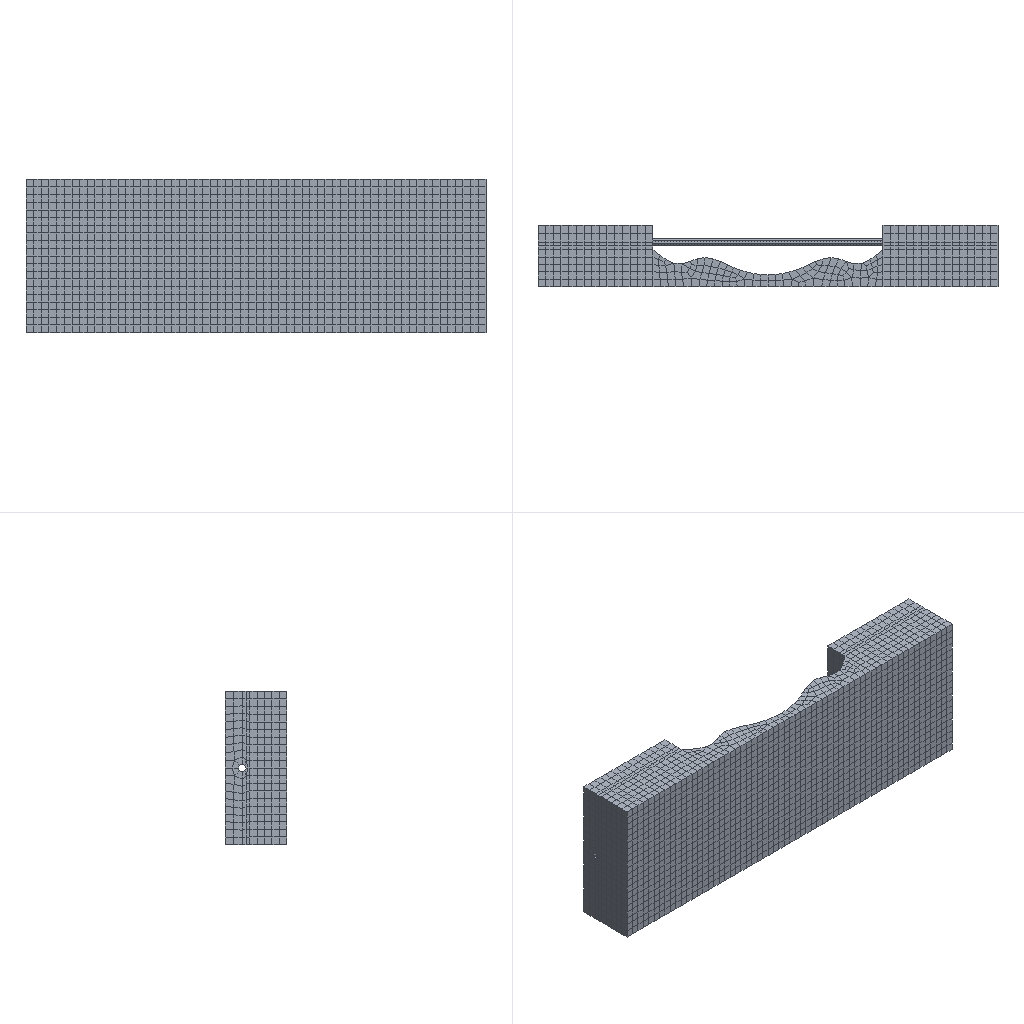Simulation study | abaqus
Set-up summary:
category,name,step,type,value,unit,region
solver,abaqus
solver,version,,,Abaqus/Standard 2020
units,not stated in the deck,,not stated
analysis,deck,,static,static
load_step,Step-G,Step-G,static,nlgeom=True
load_step,Step-2,Step-2,static,nlgeom=True
load_step,Step-3,Step-3,static,nlgeom=True
load_step,Step-4,Step-4,static,nlgeom=True
contact,interactions,,,general=1 pairs=0 ties=0
load_step,requested,,,4
mesh,nodes,,,11095
mesh,elements,,,9024
element_type,S4R,,shell,1224
element_type,C3D8R,,solid,7800
load,load commands in deck,,count,5
bc,support commands in deck,,count,4
material,GUANDAO,,in results
material,HAI,,in results
check,setup vs results,,match,"per instance, exact: element labels, types and connectivity; labels of the nodes the elements use; coordinates not compared"
Abaqus input file, long lists of numbers shortened:
*Heading
** Job name: Job-1 Model name: Model-1
** Generated by: Abaqus/CAE 2020
*Preprint, echo=NO, model=NO, history=NO, contact=NO
**
** PARTS
**
*Part, name=guan-final
*Node
      1, -0.1118, -0.2236,          30.
      2,  -0.2372, -0.07906,          30.
** (1230 more lines like these left out)
*Element, type=S4R
   1,    8,    1,    9,   16
   2,    1,    2,   10,    9
** (1222 more lines like these left out)
*Nset, nset=Set-1, generate
    1,  1232,     1
*Elset, elset=Set-1, generate
    1,  1224,     1
** Section: guandao
*Shell Section, elset=Set-1, material=guandao
0.01, 5
*End Part
**
*Part, name=merge
*Node
      1,          7.5,           0.,           5.
      2,          15.,           0.,           5.
** (9861 more lines like these left out)
*Element, type=C3D8R
  1, 1155,   96, 1141, 5340,   81,    1,   82, 1015
  2, 5340, 1141, 1142, 5341, 1015,   82,   83, 1016
** (7798 more lines like these left out)
*Nset, nset=Set-1, generate
    1,  9863,     1
*Elset, elset=Set-1, generate
    1,  7800,     1
** Section: haichuang
*Solid Section, elset=Set-1, material=hai
,
*End Part
**
**
** ASSEMBLY
**
*Assembly, name=Assembly
**
*Instance, name=merge-1, part=merge
*End Instance
**
*Instance, name=guan-final-1, part=guan-final
        -15.,          0.5,           5.
        -15.,          0.5,           5.,         -15., 1.5,           5., 90.
*End Instance
**
*Nset, nset=Set-1, instance=merge-1
   19,   20,   21,   22,   39,   42,   43,   46,   49,   50,   61,   62,   68,   72,  265,  266
  267,  268,  269,  270,  271,  272,  273,  274,  275,  276,  277,  278,  279,  280,  281,  282
** (79 more lines like these left out)
*Elset, elset=Set-1, instance=merge-1
  631,  632,  633,  634,  635,  636,  637,  638,  639,  640,  641,  642,  643,  644,  645,  646
  647,  648,  649,  650,  651,  652,  653,  654,  655,  656,  657,  658,  659,  660,  661,  662
** (73 more lines like these left out)
*Nset, nset=Set-2, instance=guan-final-1
    1,    2,    3,    4,    5,    6,    7,    8, 1225, 1226, 1227, 1228, 1229, 1230, 1231, 1232
*Elset, elset=Set-2, instance=guan-final-1
    1,    2,    3,    4,    5,    6,    7,    8, 1217, 1218, 1219, 1220, 1221, 1222, 1223, 1224
*Nset, nset=Set-3, instance=merge-1
    2,    3,    5,    9,   10,   12,   16,   17,   18,   19,   22,   25,   26,   28,   30,   31
   34,   36,   38,   41,   42,   45,   46,   48,   49,   51,   54,   56,   57,   60,   61,   64
** (26 more lines like these left out)
*Elset, elset=Set-3, instance=merge-1
   15,   16,   17,   18,   19,   20,   21,   22,   23,   24,  158,  236,  244,  252,  260,  268
  276,  284,  292,  300,  308,  337,  338,  479,  487,  488,  489,  490,  491,  492,  493,  494
** (21 more lines like these left out)
*Nset, nset=Set-4, instance=merge-1
    3,    4,    7,    9,   14,   15,   17,   18,   21,   22,   27,   28,   31,   32,   37,   38
   43,   44,   45,   46,   47,   48,   49,   50,   53,   54,   57,   58,   61,   62,   63,   64
** (56 more lines like these left out)
*Elset, elset=Set-4, instance=merge-1
   24,   33,   42,   51,   60,   69,   78,   87,   88,   89,   90,   91,   92,   93,   94,  166
  175,  184,  193,  202,  211,  220,  236,  237,  238,  239,  240,  241,  242,  243,  361,  370
** (46 more lines like these left out)
*Elset, elset=_Surf-3_SNEG, internal, instance=guan-final-1, generate
    1,  1224,     1
*Surface, type=ELEMENT, name=Surf-3
_Surf-3_SNEG, SNEG
*Elset, elset=_Surf-4_S3, internal, instance=merge-1
    1,   16,   17,   18,   19,   20,   21,   22,   23,   24,   88,   89,   90,   91,   92,   93
   94,  151,  152,  153,  154,  155,  156,  157,  158,  159,  166,  175,  184,  193,  202,  211
** (52 more lines like these left out)
*Elset, elset=_Surf-4_S4, internal, instance=merge-1
   15,   24,   33,   42,   51,   60,   69,   78,   87,   94,  101,  108,  115,  122,  129,  136
  143,  150,  158,  159,  160,  161,  162,  163,  164,  165,  229,  230,  231,  232,  233,  234
** (50 more lines like these left out)
*Elset, elset=_Surf-4_S2, internal, instance=merge-1
  166,  167,  168,  169,  170,  171,  172,  173,  174,  229,  236,  237,  238,  239,  240,  241
  242,  243,  346,  353,  354,  355,  356,  357,  358,  359,  360,  361,  416,  417,  418,  419
** (52 more lines like these left out)
*Elset, elset=_Surf-4_S6, internal, instance=merge-1
  631,  646,  661,  676,  691,  706,  721,  736,  751,  766,  781,  796,  811,  826,  841,  856
  871,  886,  901,  916,  931,  946,  961,  976,  991, 1006, 1021, 1036, 1051, 1066, 1081, 1096
** (44 more lines like these left out)
*Elset, elset=_Surf-4_S5, internal, instance=merge-1
  766,  767,  768,  769,  770,  771,  772,  773,  774,  775,  776,  777,  778,  779,  780,  916
  917,  918,  919,  920,  921,  922,  923,  924,  925,  926,  927,  928,  929,  930, 1066, 1067
** (32 more lines like these left out)
*Elset, elset=_Surf-4_S1, internal, instance=merge-1
 3436, 3437, 3438, 3439, 3440, 3441, 3442, 3443, 3444, 3445, 3446, 3447, 3448, 3449, 3450, 3451
 3452, 3453, 3454, 3455, 3456, 3457, 3458, 3459, 3460, 3461, 3462, 3463, 3464, 3465, 3466, 3467
** (10 more lines like these left out)
*Elset, elset=_Surf-4_SPOS, internal, instance=guan-final-1, generate
    1,  1224,     1
*Surface, type=ELEMENT, name=Surf-4
_Surf-4_S3, S3
_Surf-4_S4, S4
_Surf-4_S2, S2
_Surf-4_S6, S6
_Surf-4_S5, S5
_Surf-4_SPOS, SPOS
_Surf-4_S1, S1
*Elset, elset=_Surf-5_S3, internal, instance=merge-1
    1,   16,   17,   18,   19,   20,   21,   22,   23,   24,   88,   89,   90,   91,   92,   93
   94,  151,  152,  153,  154,  155,  156,  157,  158,  159,  166,  175,  184,  193,  202,  211
** (52 more lines like these left out)
*Elset, elset=_Surf-5_S4, internal, instance=merge-1
   15,   24,   33,   42,   51,   60,   69,   78,   87,   94,  101,  108,  115,  122,  129,  136
  143,  150,  158,  159,  160,  161,  162,  163,  164,  165,  229,  230,  231,  232,  233,  234
** (50 more lines like these left out)
*Elset, elset=_Surf-5_S2, internal, instance=merge-1
  166,  167,  168,  169,  170,  171,  172,  173,  174,  229,  236,  237,  238,  239,  240,  241
  242,  243,  346,  353,  354,  355,  356,  357,  358,  359,  360,  361,  416,  417,  418,  419
** (52 more lines like these left out)
*Elset, elset=_Surf-5_S6, internal, instance=merge-1
  631,  646,  661,  676,  691,  706,  721,  736,  751,  766,  781,  796,  811,  826,  841,  856
  871,  886,  901,  916,  931,  946,  961,  976,  991, 1006, 1021, 1036, 1051, 1066, 1081, 1096
** (44 more lines like these left out)
*Elset, elset=_Surf-5_S5, internal, instance=merge-1
  766,  767,  768,  769,  770,  771,  772,  773,  774,  775,  776,  777,  778,  779,  780,  916
  917,  918,  919,  920,  921,  922,  923,  924,  925,  926,  927,  928,  929,  930, 1066, 1067
** (32 more lines like these left out)
*Elset, elset=_Surf-5_S1, internal, instance=merge-1
 3436, 3437, 3438, 3439, 3440, 3441, 3442, 3443, 3444, 3445, 3446, 3447, 3448, 3449, 3450, 3451
 3452, 3453, 3454, 3455, 3456, 3457, 3458, 3459, 3460, 3461, 3462, 3463, 3464, 3465, 3466, 3467
** (10 more lines like these left out)
*Elset, elset=_Surf-5_SPOS, internal, instance=guan-final-1, generate
    1,  1224,     1
*Surface, type=ELEMENT, name=Surf-5
_Surf-5_S3, S3
_Surf-5_S4, S4
_Surf-5_S2, S2
_Surf-5_S6, S6
_Surf-5_S5, S5
_Surf-5_SPOS, SPOS
_Surf-5_S1, S1
*Elset, elset=_Surf-6_SPOS, internal, instance=guan-final-1, generate
    1,  1224,     1
*Surface, type=ELEMENT, name=Surf-6
_Surf-6_SPOS, SPOS
*Elset, elset=_m_Surf-1_SPOS, internal, instance=guan-final-1, generate
    1,  1224,     1
*Surface, type=ELEMENT, name=m_Surf-1
_m_Surf-1_SPOS, SPOS
*Elset, elset=_s_Surf-1_S3, internal, instance=merge-1
  151,  152,  153,  154,  155,  156,  157,  158,  316,  317,  318,  319,  320,  321,  322,  346
  347,  348,  349,  350,  351,  352, 1397, 1398, 1399, 1400, 1401, 1402, 1403, 1626, 1627, 1628
** (3 more lines like these left out)
*Elset, elset=_s_Surf-1_S4, internal, instance=merge-1
  159,  160,  161,  162,  163,  164,  165,  229,  230,  231,  232,  233,  234,  235,  308,  309
  310,  311,  312,  313,  314,  315,  338,  339,  340,  341,  342,  343,  344,  345, 1389, 1390
** (5 more lines like these left out)
*Elset, elset=_s_Surf-1_S2, internal, instance=merge-1
  479,  480,  481,  482,  483,  484,  485,  486, 1846, 1847, 1848, 1849, 1850, 1851, 1852, 1853
 1854, 1855, 1856, 1857, 1858, 1859, 1860, 3661, 3662, 3663, 3664, 3665, 3666, 3667, 3668, 3669
** (3 more lines like these left out)
*Surface, type=ELEMENT, name=s_Surf-1
_s_Surf-1_S3, S3
_s_Surf-1_S4, S4
_s_Surf-1_S2, S2
*Elset, elset=__Int-2_gcs0_4_S3, internal, instance=merge-1, generate
 151,  158,    1
*Elset, elset=__Int-2_gcs0_4_S4, internal, instance=merge-1
 159, 160, 161, 162, 163, 164, 165, 229, 230, 231, 232, 233, 234, 235, 308, 309
 310, 311, 312, 313, 314, 315
*Surface, type=ELEMENT, name=_Int-2_gcs0_4, internal
__Int-2_gcs0_4_S3, S3
__Int-2_gcs0_4_S4, S4
*Elset, elset=__Int-2_gcs0_12_S4, internal, instance=merge-1
 1389, 1390, 1391, 1392, 1393, 1394, 1395, 1396, 1555, 1556, 1557, 1558, 1559, 1560, 1561, 1562
*Elset, elset=__Int-2_gcs0_12_S3, internal, instance=merge-1
 1397, 1398, 1399, 1400, 1401, 1402, 1403, 1626, 1627, 1628, 1629, 1630, 1631, 1632
*Surface, type=ELEMENT, name=_Int-2_gcs0_12, internal
__Int-2_gcs0_12_S4, S4
__Int-2_gcs0_12_S3, S3
*Elset, elset=__Int-2_gcs0_22_S4, internal, instance=merge-1
 4291, 4292, 4293, 4294, 4295, 4296, 4297, 4369, 4370, 4371, 4372, 4373, 4374, 4375, 4448, 4449
 4450, 4451, 4452, 4453, 4454, 4455
*Elset, elset=__Int-2_gcs0_22_S3, internal, instance=merge-1, generate
 4298,  4305,     1
*Surface, type=ELEMENT, name=_Int-2_gcs0_22, internal
__Int-2_gcs0_22_S4, S4
__Int-2_gcs0_22_S3, S3
*Elset, elset=__Int-2_gcs0_26_S4, internal, instance=merge-1, generate
 1696,  1703,     1
*Elset, elset=__Int-2_gcs0_26_S3, internal, instance=merge-1, generate
 1704,  1710,     1
*Elset, elset=__Int-2_gcs0_26_S2, internal, instance=merge-1, generate
 1846,  1860,     1
*Surface, type=ELEMENT, name=_Int-2_gcs0_26, internal
__Int-2_gcs0_26_S4, S4
__Int-2_gcs0_26_S3, S3
__Int-2_gcs0_26_S2, S2
*Elset, elset=__Int-2_gcs0_36_S3, internal, instance=merge-1
 316, 317, 318, 319, 320, 321, 322, 346, 347, 348, 349, 350, 351, 352
*Elset, elset=__Int-2_gcs0_36_S4, internal, instance=merge-1, generate
 338,  345,    1
*Elset, elset=__Int-2_gcs0_36_S2, internal, instance=merge-1, generate
 479,  486,    1
*Surface, type=ELEMENT, name=_Int-2_gcs0_36, internal
__Int-2_gcs0_36_S3, S3
__Int-2_gcs0_36_S4, S4
__Int-2_gcs0_36_S2, S2
*Elset, elset=__Int-2_gcs0_40_S3, internal, instance=merge-1, generate
 5206,  5212,     1
*Elset, elset=__Int-2_gcs0_40_S4, internal, instance=merge-1, generate
 5213,  5220,     1
*Elset, elset=__Int-2_gcs0_40_S2, internal, instance=merge-1, generate
 5236,  5250,     1
*Surface, type=ELEMENT, name=_Int-2_gcs0_40, internal
__Int-2_gcs0_40_S3, S3
__Int-2_gcs0_40_S4, S4
__Int-2_gcs0_40_S2, S2
*Elset, elset=__Int-2_gcs0_51_S3, internal, instance=merge-1, generate
 3511,  3517,     1
*Elset, elset=__Int-2_gcs0_51_S4, internal, instance=merge-1, generate
 3518,  3525,     1
*Elset, elset=__Int-2_gcs0_51_S2, internal, instance=merge-1, generate
 3661,  3675,     1
*Surface, type=ELEMENT, name=_Int-2_gcs0_51, internal
__Int-2_gcs0_51_S3, S3
__Int-2_gcs0_51_S4, S4
__Int-2_gcs0_51_S2, S2
*Elset, elset=__Int-2_gcs0_52_S4, internal, instance=merge-1, generate
 4096,  4103,     1
*Elset, elset=__Int-2_gcs0_52_S3, internal, instance=merge-1, generate
 4104,  4110,     1
*Elset, elset=__Int-2_gcs0_52_S2, internal, instance=merge-1, generate
 4111,  4125,     1
*Surface, type=ELEMENT, name=_Int-2_gcs0_52, internal
__Int-2_gcs0_52_S4, S4
__Int-2_gcs0_52_S3, S3
__Int-2_gcs0_52_S2, S2
*Elset, elset=__Int-2_gcs0_69_S4, internal, instance=merge-1
 5526, 5527, 5529, 5546, 5581, 5640, 5641, 5643, 5660, 5695, 5754, 5755, 5757, 5774, 5809, 5868
 5869, 5871, 5888, 5923, 5982, 5983, 5985, 6002, 6037, 6096, 6097, 6099, 6116, 6151, 6210, 6211
** (5 more lines like these left out)
*Elset, elset=__Int-2_gcs0_69_S6, internal, instance=merge-1
 5530, 5531, 5542, 5543, 5545, 5578, 5584, 5644, 5645, 5656, 5657, 5659, 5692, 5698, 5758, 5759
 5770, 5771, 5773, 5806, 5812, 5872, 5873, 5884, 5885, 5887, 5920, 5926, 5986, 5987, 5998, 5999
** (7 more lines like these left out)
*Surface, type=ELEMENT, name=_Int-2_gcs0_69, internal
__Int-2_gcs0_69_S4, S4
__Int-2_gcs0_69_S6, S6
*Elset, elset=__Int-2_gcs0_73_SPOS, internal, instance=guan-final-1, generate
    1,  1224,     1
*Surface, type=ELEMENT, name=_Int-2_gcs0_73, internal
__Int-2_gcs0_73_SPOS, SPOS
*Elset, elset=__Int-2_gcs0_74_SNEG, internal, instance=guan-final-1, generate
    1,  1224,     1
*Surface, type=ELEMENT, name=_Int-2_gcs0_74, internal
__Int-2_gcs0_74_SNEG, SNEG
*End Assembly
*Amplitude, name=Amp-1
             0.,              0.,              1.,              1.
**
** MATERIALS
**
*Material, name=guandao
*Density
7800.,
*Elastic
 2.07e+11, 0.3
*Plastic
 3.6e+08,       0.
 3.8e+08, 0.002676
   4e+08, 0.004728
 4.2e+08, 0.008045
 4.4e+08,  0.01332
 4.6e+08,  0.02158
 4.8e+08,  0.03427
*Material, name=hai
*Density
2000.,
*Elastic
 1.05e+07, 0.3
*Mohr Coulomb
25.,22.
*Mohr Coulomb Hardening
 5e+06,0.
**
** INTERACTION PROPERTIES
**
*Surface Interaction, name=IntProp-1
1.,
*Friction, slip tolerance=0.005
 0.5,
*Surface Behavior, pressure-overclosure=HARD
**
** INTERACTIONS
**
** Interaction: Int-2
*Contact
*Contact Inclusions, ALL EXTERIOR
*Contact Property Assignment
 ,  , IntProp-1
*Surface Property Assignment, property=GEOMETRIC CORRECTION
_Int-2_gcs0_4, Circumferential, -15., 0.5, 5.,  -14., 0.5, 5.
_Int-2_gcs0_12, Circumferential, -15., 0.5, 5.,  -14., 0.5, 5.
_Int-2_gcs0_22, Circumferential, -15., 0.5, 5.,  -14., 0.5, 5.
_Int-2_gcs0_26, Circumferential, -15., 0.5, 5.,  -14., 0.5, 5.
_Int-2_gcs0_36, Circumferential, -15., 0.5, 5.,  -14., 0.5, 5.
_Int-2_gcs0_40, Circumferential, -15., 0.5, 5.,  -14., 0.5, 5.
_Int-2_gcs0_51, Circumferential, -15., 0.5, 5.,  -14., 0.5, 5.
_Int-2_gcs0_52, Circumferential, -15., 0.5, 5.,  -14., 0.5, 5.
_Int-2_gcs0_69, Circumferential, 0., 3.96, 0.,  0., 3.96, 1.
_Int-2_gcs0_73, Circumferential, -15., 0.5, 5.,  -14., 0.5, 5.
_Int-2_gcs0_74, Circumferential, -15., 0.5, 5.,  -14., 0.5, 5.
** ----------------------------------------------------------------
**
** STEP: Step-G
**
*Step, name=Step-G, nlgeom=YES, inc=1000
*Static, stabilize=0.0002, allsdtol=0.05, continue=NO
0.01, 1., 1e-05, 1.
**
** BOUNDARY CONDITIONS
**
** Name: BC-1 Type: 位移/转角
*Boundary
Set-1, 2, 2
** Name: BC-2 Type: 位移/转角
*Boundary
Set-2, 1, 1
** Name: BC-3 Type: 位移/转角
*Boundary
Set-3, 1, 1
** Name: BC-4 Type: 位移/转角
*Boundary
Set-4, 3, 3
**
** LOADS
**
** Name: Load-1   Type: Gravity
*Dload
, GRAV, 100., 0., -1., 0.
**
** OUTPUT REQUESTS
**
*Restart, write, frequency=0
**
** FIELD OUTPUT: F-Output-1
**
*Output, field, variable=PRESELECT
**
** HISTORY OUTPUT: H-Output-1
**
*Output, history, variable=PRESELECT
*End Step
** ----------------------------------------------------------------
**
** STEP: Step-2
**
*Step, name=Step-2, nlgeom=YES, inc=1000
*Static, stabilize=0.0002, allsdtol=0.05, continue=NO
0.01, 1., 1e-05, 1.
**
** LOADS
**
** Name: Load-guanzhouxiang   Type: Surface traction
*Dsload, amplitude=Amp-1
Surf-6, TRVEC, 200., -1., 0., 4.73695e-16
** Name: Load-p   Type: Pressure
*Dsload, amplitude=Amp-1
Surf-3, P, 1e+06
**
** OUTPUT REQUESTS
**
*Restart, write, frequency=0
**
** FIELD OUTPUT: F-Output-1
**
*Output, field
*Node Output
CF, RF, TF, U, V
*Element Output, directions=YES
E, LE, MISES, MISESMAX, PE, PEEQ, PEMAG, S, SF, SSAVG
*Contact Output
CDISP, CSTRESS
**
** HISTORY OUTPUT: H-Output-1
**
*Output, history, variable=PRESELECT
*End Step
** ----------------------------------------------------------------
**
** STEP: Step-3
**
*Step, name=Step-3, nlgeom=YES, inc=1000
*Static, stabilize=0.0002, allsdtol=0.05, continue=NO
0.01, 1., 1e-05, 1.
**
** LOADS
**
** Name: Load-hengxiang   Type: Surface traction
*Dsload, amplitude=Amp-1
Surf-4, TRVEC, 400., 1., 0., 4.73695e-16
**
** OUTPUT REQUESTS
**
*Restart, write, frequency=0
**
** FIELD OUTPUT: F-Output-1
**
*Output, field
*Node Output
CF, RF, TF, U, V
*Element Output, directions=YES
E, LE, MISES, MISESMAX, PE, PEEQ, PEMAG, S, SF, SSAVG
*Contact Output
CDISP, CSTRESS
**
** HISTORY OUTPUT: H-Output-1
**
*Output, history, variable=PRESELECT
*End Step
** ----------------------------------------------------------------
**
** STEP: Step-4
**
*Step, name=Step-4, nlgeom=YES, inc=1000
*Static, stabilize=0.0002, allsdtol=0.05, continue=NO
0.01, 1., 1e-05, 1.
**
** LOADS
**
** Name: Load-zongxiangli   Type: Surface traction
*Dsload, amplitude=Amp-1
Surf-5, TRVEC, 500., 0., 0., -1.
**
** OUTPUT REQUESTS
**
*Restart, write, frequency=0
**
** FIELD OUTPUT: F-Output-1
**
*Output, field
*Node Output
CF, RF, TF, U, V
*Element Output, directions=YES
E, LE, MISES, MISESMAX, PE, PEEQ, PEMAG, S, SF, SSAVG
*Contact Output
CDISP, CSTRESS
**
** HISTORY OUTPUT: H-Output-1
**
*Output, history, variable=PRESELECT
*End Step
Results summary:
result,step,,completed,increments=14 time=1.0/1.0
result,step,,completed,increments=11 time=1.0/1.0
result,step,,completed,increments=11 time=1.0/1.0
result,step,,completed,increments=12 time=1.0/1.0
result,analysis,,,static
result,last_loadstep,,,4
result,analysis steps,,count,4
result,primary field,,,"U, UR"
result,reaction total,,FX,-369385.958,model units
result,reaction total,,FY,164107440.543,model units
result,reaction total,,FZ,471118.337,model units